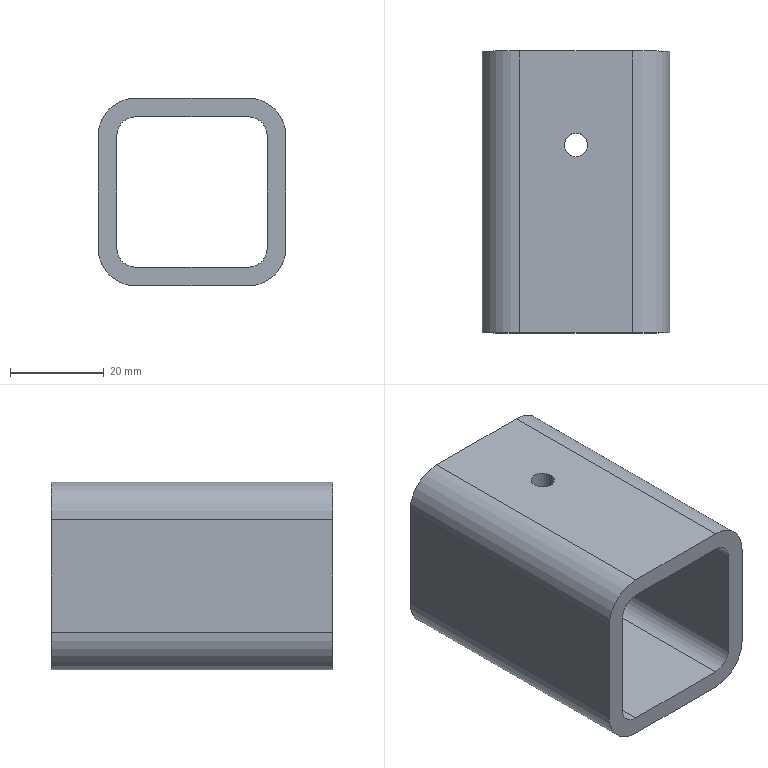Part | SolidWorks | features HoleWzd 1, WeldMemberFeat 1, WeldmentFeature 1 | 1 solid | 22 faces | box 40 x 60 x 40 mm | volume 31931 mm3 | cylinder 12 | plane 10 | commonest cylinder face diameters 5 x4 8 x4 16 x4
STEP:
#1=CARTESIAN_POINT('',(2.5,40.,16.));
#2=VERTEX_POINT('',#1);
#3=CARTESIAN_POINT('',(-2.5,40.,16.));
#4=VERTEX_POINT('',#3);
#5=CARTESIAN_POINT('',(0.,40.,16.));
#6=DIRECTION('',(0.,0.,-1.));
#7=DIRECTION('',(-1.,0.,0.));
#8=AXIS2_PLACEMENT_3D('',#5,#6,#7);
#9=CIRCLE('',#8,2.5);
#10=EDGE_CURVE('',#2,#4,#9,.T.);
#11=ORIENTED_EDGE('',*,*,#10,.T.);
#12=CARTESIAN_POINT('',(-2.5,40.,20.));
#13=VERTEX_POINT('',#12);
#14=CARTESIAN_POINT('',(-2.5,40.,20.));
#15=DIRECTION('',(0.,0.,1.));
#16=VECTOR('',#15,1000.);
#17=LINE('',#14,#16);
#18=EDGE_CURVE('',#4,#13,#17,.T.);
#19=ORIENTED_EDGE('',*,*,#18,.T.);
#20=CARTESIAN_POINT('',(2.5,40.,20.));
#21=VERTEX_POINT('',#20);
#22=CARTESIAN_POINT('',(0.,40.,20.));
#23=DIRECTION('',(0.,0.,1.));
#24=DIRECTION('',(1.,0.,0.));
#25=AXIS2_PLACEMENT_3D('',#22,#23,#24);
#26=CIRCLE('',#25,2.5);
#27=EDGE_CURVE('',#13,#21,#26,.T.);
#28=ORIENTED_EDGE('',*,*,#27,.T.);
#29=CARTESIAN_POINT('',(2.5,40.,20.));
#30=DIRECTION('',(0.,0.,1.));
#31=VECTOR('',#30,1000.);
#32=LINE('',#29,#31);
#33=EDGE_CURVE('',#2,#21,#32,.T.);
#34=ORIENTED_EDGE('',*,*,#33,.F.);
#35=EDGE_LOOP('',(#11,#19,#28,#34));
#36=FACE_OUTER_BOUND('',#35,.T.);
#37=CARTESIAN_POINT('',(0.,40.,20.));
#38=DIRECTION('',(0.,0.,1.));
#39=DIRECTION('',(1.,0.,0.));
#40=AXIS2_PLACEMENT_3D('',#37,#38,#39);
#41=CYLINDRICAL_SURFACE('',#40,2.5);
#42=ADVANCED_FACE('',(#36),#41,.F.);
#43=CARTESIAN_POINT('',(-2.5,40.,-20.));
#44=VERTEX_POINT('',#43);
#45=CARTESIAN_POINT('',(2.5,40.,-20.));
#46=VERTEX_POINT('',#45);
#47=CARTESIAN_POINT('',(0.,40.,-20.));
#48=DIRECTION('',(0.,0.,1.));
#49=DIRECTION('',(1.,0.,0.));
#50=AXIS2_PLACEMENT_3D('',#47,#48,#49);
#51=CIRCLE('',#50,2.5);
#52=EDGE_CURVE('',#44,#46,#51,.T.);
#53=ORIENTED_EDGE('',*,*,#52,.F.);
#54=CARTESIAN_POINT('',(-2.5,40.,-16.));
#55=VERTEX_POINT('',#54);
#56=CARTESIAN_POINT('',(-2.5,40.,20.));
#57=DIRECTION('',(0.,0.,1.));
#58=VECTOR('',#57,1000.);
#59=LINE('',#56,#58);
#60=EDGE_CURVE('',#44,#55,#59,.T.);
#61=ORIENTED_EDGE('',*,*,#60,.T.);
#62=CARTESIAN_POINT('',(2.5,40.,-16.));
#63=VERTEX_POINT('',#62);
#64=CARTESIAN_POINT('',(0.,40.,-16.));
#65=DIRECTION('',(0.,0.,1.));
#66=DIRECTION('',(1.,0.,0.));
#67=AXIS2_PLACEMENT_3D('',#64,#65,#66);
#68=CIRCLE('',#67,2.5);
#69=EDGE_CURVE('',#55,#63,#68,.T.);
#70=ORIENTED_EDGE('',*,*,#69,.T.);
#71=CARTESIAN_POINT('',(2.5,40.,20.));
#72=DIRECTION('',(0.,0.,1.));
#73=VECTOR('',#72,1000.);
#74=LINE('',#71,#73);
#75=EDGE_CURVE('',#46,#63,#74,.T.);
#76=ORIENTED_EDGE('',*,*,#75,.F.);
#77=EDGE_LOOP('',(#53,#61,#70,#76));
#78=FACE_OUTER_BOUND('',#77,.T.);
#79=CARTESIAN_POINT('',(0.,40.,20.));
#80=DIRECTION('',(0.,0.,1.));
#81=DIRECTION('',(1.,0.,0.));
#82=AXIS2_PLACEMENT_3D('',#79,#80,#81);
#83=CYLINDRICAL_SURFACE('',#82,2.5);
#84=ADVANCED_FACE('',(#78),#83,.F.);
#85=CARTESIAN_POINT('',(20.,60.,12.));
#86=VERTEX_POINT('',#85);
#87=CARTESIAN_POINT('',(12.,60.,20.));
#88=VERTEX_POINT('',#87);
#89=CARTESIAN_POINT('',(12.,60.,12.));
#90=DIRECTION('',(0.,-1.,0.));
#91=DIRECTION('',(1.,0.,0.));
#92=AXIS2_PLACEMENT_3D('',#89,#90,#91);
#93=CIRCLE('',#92,8.);
#94=EDGE_CURVE('',#86,#88,#93,.T.);
#95=ORIENTED_EDGE('',*,*,#94,.T.);
#96=CARTESIAN_POINT('',(12.,0.,20.));
#97=VERTEX_POINT('',#96);
#98=CARTESIAN_POINT('',(12.,0.,20.));
#99=DIRECTION('',(0.,1.,0.));
#100=VECTOR('',#99,1000.);
#101=LINE('',#98,#100);
#102=EDGE_CURVE('',#97,#88,#101,.T.);
#103=ORIENTED_EDGE('',*,*,#102,.F.);
#104=CARTESIAN_POINT('',(20.,0.,12.));
#105=VERTEX_POINT('',#104);
#106=CARTESIAN_POINT('',(12.,0.,12.));
#107=DIRECTION('',(0.,-1.,0.));
#108=DIRECTION('',(1.,0.,0.));
#109=AXIS2_PLACEMENT_3D('',#106,#107,#108);
#110=CIRCLE('',#109,8.);
#111=EDGE_CURVE('',#105,#97,#110,.T.);
#112=ORIENTED_EDGE('',*,*,#111,.F.);
#113=CARTESIAN_POINT('',(20.,0.,12.));
#114=DIRECTION('',(0.,1.,0.));
#115=VECTOR('',#114,1000.);
#116=LINE('',#113,#115);
#117=EDGE_CURVE('',#105,#86,#116,.T.);
#118=ORIENTED_EDGE('',*,*,#117,.T.);
#119=EDGE_LOOP('',(#95,#103,#112,#118));
#120=FACE_OUTER_BOUND('',#119,.T.);
#121=CARTESIAN_POINT('',(12.,0.,12.));
#122=DIRECTION('',(0.,1.,0.));
#123=DIRECTION('',(-1.,0.,0.));
#124=AXIS2_PLACEMENT_3D('',#121,#122,#123);
#125=CYLINDRICAL_SURFACE('',#124,8.);
#126=ADVANCED_FACE('',(#120),#125,.T.);
#127=CARTESIAN_POINT('',(0.,40.,20.));
#128=DIRECTION('',(0.,0.,1.));
#129=DIRECTION('',(1.,0.,0.));
#130=AXIS2_PLACEMENT_3D('',#127,#128,#129);
#131=CIRCLE('',#130,2.5);
#132=EDGE_CURVE('',#21,#13,#131,.T.);
#133=ORIENTED_EDGE('',*,*,#132,.F.);
#134=ORIENTED_EDGE('',*,*,#27,.F.);
#135=EDGE_LOOP('',(#133,#134));
#136=FACE_BOUND('',#135,.T.);
#137=CARTESIAN_POINT('',(-12.,60.,20.));
#138=VERTEX_POINT('',#137);
#139=CARTESIAN_POINT('',(12.,60.,20.));
#140=DIRECTION('',(-1.,0.,0.));
#141=VECTOR('',#140,1000.);
#142=LINE('',#139,#141);
#143=EDGE_CURVE('',#88,#138,#142,.T.);
#144=ORIENTED_EDGE('',*,*,#143,.T.);
#145=CARTESIAN_POINT('',(-12.,0.,20.));
#146=VERTEX_POINT('',#145);
#147=CARTESIAN_POINT('',(-12.,0.,20.));
#148=DIRECTION('',(0.,1.,0.));
#149=VECTOR('',#148,1000.);
#150=LINE('',#147,#149);
#151=EDGE_CURVE('',#146,#138,#150,.T.);
#152=ORIENTED_EDGE('',*,*,#151,.F.);
#153=CARTESIAN_POINT('',(12.,0.,20.));
#154=DIRECTION('',(-1.,0.,0.));
#155=VECTOR('',#154,1000.);
#156=LINE('',#153,#155);
#157=EDGE_CURVE('',#97,#146,#156,.T.);
#158=ORIENTED_EDGE('',*,*,#157,.F.);
#159=ORIENTED_EDGE('',*,*,#102,.T.);
#160=EDGE_LOOP('',(#144,#152,#158,#159));
#161=FACE_OUTER_BOUND('',#160,.T.);
#162=CARTESIAN_POINT('',(12.,0.,20.));
#163=DIRECTION('',(0.,0.,-1.));
#164=DIRECTION('',(-1.,0.,0.));
#165=AXIS2_PLACEMENT_3D('',#162,#163,#164);
#166=PLANE('',#165);
#167=ADVANCED_FACE('',(#136,#161),#166,.F.);
#168=CARTESIAN_POINT('',(-20.,60.,12.));
#169=VERTEX_POINT('',#168);
#170=CARTESIAN_POINT('',(-12.,60.,12.));
#171=DIRECTION('',(0.,-1.,0.));
#172=DIRECTION('',(1.,0.,0.));
#173=AXIS2_PLACEMENT_3D('',#170,#171,#172);
#174=CIRCLE('',#173,8.);
#175=EDGE_CURVE('',#138,#169,#174,.T.);
#176=ORIENTED_EDGE('',*,*,#175,.T.);
#177=CARTESIAN_POINT('',(-20.,0.,12.));
#178=VERTEX_POINT('',#177);
#179=CARTESIAN_POINT('',(-20.,0.,12.));
#180=DIRECTION('',(0.,1.,0.));
#181=VECTOR('',#180,1000.);
#182=LINE('',#179,#181);
#183=EDGE_CURVE('',#178,#169,#182,.T.);
#184=ORIENTED_EDGE('',*,*,#183,.F.);
#185=CARTESIAN_POINT('',(-12.,0.,12.));
#186=DIRECTION('',(0.,-1.,0.));
#187=DIRECTION('',(1.,0.,0.));
#188=AXIS2_PLACEMENT_3D('',#185,#186,#187);
#189=CIRCLE('',#188,8.);
#190=EDGE_CURVE('',#146,#178,#189,.T.);
#191=ORIENTED_EDGE('',*,*,#190,.F.);
#192=ORIENTED_EDGE('',*,*,#151,.T.);
#193=EDGE_LOOP('',(#176,#184,#191,#192));
#194=FACE_OUTER_BOUND('',#193,.T.);
#195=CARTESIAN_POINT('',(-12.,0.,12.));
#196=DIRECTION('',(0.,1.,0.));
#197=DIRECTION('',(-1.,0.,0.));
#198=AXIS2_PLACEMENT_3D('',#195,#196,#197);
#199=CYLINDRICAL_SURFACE('',#198,8.);
#200=ADVANCED_FACE('',(#194),#199,.T.);
#201=CARTESIAN_POINT('',(-20.,60.,-12.));
#202=VERTEX_POINT('',#201);
#203=CARTESIAN_POINT('',(-20.,60.,-12.));
#204=DIRECTION('',(0.,0.,-1.));
#205=VECTOR('',#204,1000.);
#206=LINE('',#203,#205);
#207=EDGE_CURVE('',#169,#202,#206,.T.);
#208=ORIENTED_EDGE('',*,*,#207,.T.);
#209=CARTESIAN_POINT('',(-20.,0.,-12.));
#210=VERTEX_POINT('',#209);
#211=CARTESIAN_POINT('',(-20.,0.,-12.));
#212=DIRECTION('',(0.,1.,0.));
#213=VECTOR('',#212,1000.);
#214=LINE('',#211,#213);
#215=EDGE_CURVE('',#210,#202,#214,.T.);
#216=ORIENTED_EDGE('',*,*,#215,.F.);
#217=CARTESIAN_POINT('',(-20.,0.,-12.));
#218=DIRECTION('',(0.,0.,-1.));
#219=VECTOR('',#218,1000.);
#220=LINE('',#217,#219);
#221=EDGE_CURVE('',#178,#210,#220,.T.);
#222=ORIENTED_EDGE('',*,*,#221,.F.);
#223=ORIENTED_EDGE('',*,*,#183,.T.);
#224=EDGE_LOOP('',(#208,#216,#222,#223));
#225=FACE_OUTER_BOUND('',#224,.T.);
#226=CARTESIAN_POINT('',(-20.,0.,-12.));
#227=DIRECTION('',(1.,0.,0.));
#228=DIRECTION('',(0.,1.,0.));
#229=AXIS2_PLACEMENT_3D('',#226,#227,#228);
#230=PLANE('',#229);
#231=ADVANCED_FACE('',(#225),#230,.F.);
#232=CARTESIAN_POINT('',(-12.,60.,-20.));
#233=VERTEX_POINT('',#232);
#234=CARTESIAN_POINT('',(-12.,60.,-12.));
#235=DIRECTION('',(0.,-1.,0.));
#236=DIRECTION('',(1.,0.,0.));
#237=AXIS2_PLACEMENT_3D('',#234,#235,#236);
#238=CIRCLE('',#237,8.);
#239=EDGE_CURVE('',#202,#233,#238,.T.);
#240=ORIENTED_EDGE('',*,*,#239,.T.);
#241=CARTESIAN_POINT('',(-12.,0.,-20.));
#242=VERTEX_POINT('',#241);
#243=CARTESIAN_POINT('',(-12.,0.,-20.));
#244=DIRECTION('',(0.,1.,0.));
#245=VECTOR('',#244,1000.);
#246=LINE('',#243,#245);
#247=EDGE_CURVE('',#242,#233,#246,.T.);
#248=ORIENTED_EDGE('',*,*,#247,.F.);
#249=CARTESIAN_POINT('',(-12.,0.,-12.));
#250=DIRECTION('',(0.,-1.,0.));
#251=DIRECTION('',(1.,0.,0.));
#252=AXIS2_PLACEMENT_3D('',#249,#250,#251);
#253=CIRCLE('',#252,8.);
#254=EDGE_CURVE('',#210,#242,#253,.T.);
#255=ORIENTED_EDGE('',*,*,#254,.F.);
#256=ORIENTED_EDGE('',*,*,#215,.T.);
#257=EDGE_LOOP('',(#240,#248,#255,#256));
#258=FACE_OUTER_BOUND('',#257,.T.);
#259=CARTESIAN_POINT('',(-12.,0.,-12.));
#260=DIRECTION('',(0.,1.,0.));
#261=DIRECTION('',(-1.,0.,0.));
#262=AXIS2_PLACEMENT_3D('',#259,#260,#261);
#263=CYLINDRICAL_SURFACE('',#262,8.);
#264=ADVANCED_FACE('',(#258),#263,.T.);
#265=CARTESIAN_POINT('',(0.,40.,-20.));
#266=DIRECTION('',(0.,0.,1.));
#267=DIRECTION('',(1.,0.,0.));
#268=AXIS2_PLACEMENT_3D('',#265,#266,#267);
#269=CIRCLE('',#268,2.5);
#270=EDGE_CURVE('',#46,#44,#269,.T.);
#271=ORIENTED_EDGE('',*,*,#270,.T.);
#272=ORIENTED_EDGE('',*,*,#52,.T.);
#273=EDGE_LOOP('',(#271,#272));
#274=FACE_BOUND('',#273,.T.);
#275=CARTESIAN_POINT('',(12.,60.,-20.));
#276=VERTEX_POINT('',#275);
#277=CARTESIAN_POINT('',(-12.,60.,-20.));
#278=DIRECTION('',(1.,0.,0.));
#279=VECTOR('',#278,1000.);
#280=LINE('',#277,#279);
#281=EDGE_CURVE('',#233,#276,#280,.T.);
#282=ORIENTED_EDGE('',*,*,#281,.T.);
#283=CARTESIAN_POINT('',(12.,0.,-20.));
#284=VERTEX_POINT('',#283);
#285=CARTESIAN_POINT('',(12.,0.,-20.));
#286=DIRECTION('',(0.,1.,0.));
#287=VECTOR('',#286,1000.);
#288=LINE('',#285,#287);
#289=EDGE_CURVE('',#284,#276,#288,.T.);
#290=ORIENTED_EDGE('',*,*,#289,.F.);
#291=CARTESIAN_POINT('',(-12.,0.,-20.));
#292=DIRECTION('',(1.,0.,0.));
#293=VECTOR('',#292,1000.);
#294=LINE('',#291,#293);
#295=EDGE_CURVE('',#242,#284,#294,.T.);
#296=ORIENTED_EDGE('',*,*,#295,.F.);
#297=ORIENTED_EDGE('',*,*,#247,.T.);
#298=EDGE_LOOP('',(#282,#290,#296,#297));
#299=FACE_OUTER_BOUND('',#298,.T.);
#300=CARTESIAN_POINT('',(-12.,0.,-20.));
#301=DIRECTION('',(0.,0.,1.));
#302=DIRECTION('',(1.,0.,0.));
#303=AXIS2_PLACEMENT_3D('',#300,#301,#302);
#304=PLANE('',#303);
#305=ADVANCED_FACE('',(#274,#299),#304,.F.);
#306=CARTESIAN_POINT('',(20.,60.,-12.));
#307=VERTEX_POINT('',#306);
#308=CARTESIAN_POINT('',(12.,60.,-12.));
#309=DIRECTION('',(0.,-1.,0.));
#310=DIRECTION('',(1.,0.,0.));
#311=AXIS2_PLACEMENT_3D('',#308,#309,#310);
#312=CIRCLE('',#311,8.);
#313=EDGE_CURVE('',#276,#307,#312,.T.);
#314=ORIENTED_EDGE('',*,*,#313,.T.);
#315=CARTESIAN_POINT('',(20.,0.,-12.));
#316=VERTEX_POINT('',#315);
#317=CARTESIAN_POINT('',(20.,0.,-12.));
#318=DIRECTION('',(0.,1.,0.));
#319=VECTOR('',#318,1000.);
#320=LINE('',#317,#319);
#321=EDGE_CURVE('',#316,#307,#320,.T.);
#322=ORIENTED_EDGE('',*,*,#321,.F.);
#323=CARTESIAN_POINT('',(12.,0.,-12.));
#324=DIRECTION('',(0.,-1.,0.));
#325=DIRECTION('',(1.,0.,0.));
#326=AXIS2_PLACEMENT_3D('',#323,#324,#325);
#327=CIRCLE('',#326,8.);
#328=EDGE_CURVE('',#284,#316,#327,.T.);
#329=ORIENTED_EDGE('',*,*,#328,.F.);
#330=ORIENTED_EDGE('',*,*,#289,.T.);
#331=EDGE_LOOP('',(#314,#322,#329,#330));
#332=FACE_OUTER_BOUND('',#331,.T.);
#333=CARTESIAN_POINT('',(12.,0.,-12.));
#334=DIRECTION('',(0.,1.,0.));
#335=DIRECTION('',(-1.,0.,0.));
#336=AXIS2_PLACEMENT_3D('',#333,#334,#335);
#337=CYLINDRICAL_SURFACE('',#336,8.);
#338=ADVANCED_FACE('',(#332),#337,.T.);
#339=CARTESIAN_POINT('',(-12.,60.,16.));
#340=VERTEX_POINT('',#339);
#341=CARTESIAN_POINT('',(-16.,60.,12.));
#342=VERTEX_POINT('',#341);
#343=CARTESIAN_POINT('',(-12.,60.,12.));
#344=DIRECTION('',(0.,-1.,0.));
#345=DIRECTION('',(1.,0.,0.));
#346=AXIS2_PLACEMENT_3D('',#343,#344,#345);
#347=CIRCLE('',#346,4.);
#348=EDGE_CURVE('',#340,#342,#347,.T.);
#349=ORIENTED_EDGE('',*,*,#348,.F.);
#350=CARTESIAN_POINT('',(-12.,0.,16.));
#351=VERTEX_POINT('',#350);
#352=CARTESIAN_POINT('',(-12.,0.,16.));
#353=DIRECTION('',(0.,1.,0.));
#354=VECTOR('',#353,1000.);
#355=LINE('',#352,#354);
#356=EDGE_CURVE('',#351,#340,#355,.T.);
#357=ORIENTED_EDGE('',*,*,#356,.F.);
#358=CARTESIAN_POINT('',(-16.,0.,12.));
#359=VERTEX_POINT('',#358);
#360=CARTESIAN_POINT('',(-12.,0.,12.));
#361=DIRECTION('',(0.,-1.,0.));
#362=DIRECTION('',(1.,0.,0.));
#363=AXIS2_PLACEMENT_3D('',#360,#361,#362);
#364=CIRCLE('',#363,4.);
#365=EDGE_CURVE('',#351,#359,#364,.T.);
#366=ORIENTED_EDGE('',*,*,#365,.T.);
#367=CARTESIAN_POINT('',(-16.,0.,12.));
#368=DIRECTION('',(0.,1.,0.));
#369=VECTOR('',#368,1000.);
#370=LINE('',#367,#369);
#371=EDGE_CURVE('',#359,#342,#370,.T.);
#372=ORIENTED_EDGE('',*,*,#371,.T.);
#373=EDGE_LOOP('',(#349,#357,#366,#372));
#374=FACE_OUTER_BOUND('',#373,.T.);
#375=CARTESIAN_POINT('',(-12.,0.,12.));
#376=DIRECTION('',(0.,1.,0.));
#377=DIRECTION('',(-1.,0.,0.));
#378=AXIS2_PLACEMENT_3D('',#375,#376,#377);
#379=CYLINDRICAL_SURFACE('',#378,4.);
#380=ADVANCED_FACE('',(#374),#379,.F.);
#381=ORIENTED_EDGE('',*,*,#10,.F.);
#382=CARTESIAN_POINT('',(0.,40.,16.));
#383=DIRECTION('',(0.,0.,-1.));
#384=DIRECTION('',(-1.,0.,0.));
#385=AXIS2_PLACEMENT_3D('',#382,#383,#384);
#386=CIRCLE('',#385,2.5);
#387=EDGE_CURVE('',#4,#2,#386,.T.);
#388=ORIENTED_EDGE('',*,*,#387,.F.);
#389=EDGE_LOOP('',(#381,#388));
#390=FACE_BOUND('',#389,.T.);
#391=CARTESIAN_POINT('',(12.,60.,16.));
#392=VERTEX_POINT('',#391);
#393=CARTESIAN_POINT('',(12.,60.,16.));
#394=DIRECTION('',(-1.,0.,0.));
#395=VECTOR('',#394,1000.);
#396=LINE('',#393,#395);
#397=EDGE_CURVE('',#392,#340,#396,.T.);
#398=ORIENTED_EDGE('',*,*,#397,.F.);
#399=CARTESIAN_POINT('',(12.,0.,16.));
#400=VERTEX_POINT('',#399);
#401=CARTESIAN_POINT('',(12.,0.,16.));
#402=DIRECTION('',(0.,1.,0.));
#403=VECTOR('',#402,1000.);
#404=LINE('',#401,#403);
#405=EDGE_CURVE('',#400,#392,#404,.T.);
#406=ORIENTED_EDGE('',*,*,#405,.F.);
#407=CARTESIAN_POINT('',(12.,0.,16.));
#408=DIRECTION('',(-1.,0.,0.));
#409=VECTOR('',#408,1000.);
#410=LINE('',#407,#409);
#411=EDGE_CURVE('',#400,#351,#410,.T.);
#412=ORIENTED_EDGE('',*,*,#411,.T.);
#413=ORIENTED_EDGE('',*,*,#356,.T.);
#414=EDGE_LOOP('',(#398,#406,#412,#413));
#415=FACE_OUTER_BOUND('',#414,.T.);
#416=CARTESIAN_POINT('',(12.,0.,16.));
#417=DIRECTION('',(0.,0.,-1.));
#418=DIRECTION('',(-1.,0.,0.));
#419=AXIS2_PLACEMENT_3D('',#416,#417,#418);
#420=PLANE('',#419);
#421=ADVANCED_FACE('',(#390,#415),#420,.T.);
#422=CARTESIAN_POINT('',(16.,60.,12.));
#423=VERTEX_POINT('',#422);
#424=CARTESIAN_POINT('',(12.,60.,12.));
#425=DIRECTION('',(0.,-1.,0.));
#426=DIRECTION('',(1.,0.,0.));
#427=AXIS2_PLACEMENT_3D('',#424,#425,#426);
#428=CIRCLE('',#427,4.);
#429=EDGE_CURVE('',#423,#392,#428,.T.);
#430=ORIENTED_EDGE('',*,*,#429,.F.);
#431=CARTESIAN_POINT('',(16.,0.,12.));
#432=VERTEX_POINT('',#431);
#433=CARTESIAN_POINT('',(16.,0.,12.));
#434=DIRECTION('',(0.,1.,0.));
#435=VECTOR('',#434,1000.);
#436=LINE('',#433,#435);
#437=EDGE_CURVE('',#432,#423,#436,.T.);
#438=ORIENTED_EDGE('',*,*,#437,.F.);
#439=CARTESIAN_POINT('',(12.,0.,12.));
#440=DIRECTION('',(0.,-1.,0.));
#441=DIRECTION('',(1.,0.,0.));
#442=AXIS2_PLACEMENT_3D('',#439,#440,#441);
#443=CIRCLE('',#442,4.);
#444=EDGE_CURVE('',#432,#400,#443,.T.);
#445=ORIENTED_EDGE('',*,*,#444,.T.);
#446=ORIENTED_EDGE('',*,*,#405,.T.);
#447=EDGE_LOOP('',(#430,#438,#445,#446));
#448=FACE_OUTER_BOUND('',#447,.T.);
#449=CARTESIAN_POINT('',(12.,0.,12.));
#450=DIRECTION('',(0.,1.,0.));
#451=DIRECTION('',(-1.,0.,0.));
#452=AXIS2_PLACEMENT_3D('',#449,#450,#451);
#453=CYLINDRICAL_SURFACE('',#452,4.);
#454=ADVANCED_FACE('',(#448),#453,.F.);
#455=CARTESIAN_POINT('',(16.,60.,-12.));
#456=VERTEX_POINT('',#455);
#457=CARTESIAN_POINT('',(16.,60.,12.));
#458=DIRECTION('',(0.,0.,1.));
#459=VECTOR('',#458,1000.);
#460=LINE('',#457,#459);
#461=EDGE_CURVE('',#456,#423,#460,.T.);
#462=ORIENTED_EDGE('',*,*,#461,.F.);
#463=CARTESIAN_POINT('',(16.,0.,-12.));
#464=VERTEX_POINT('',#463);
#465=CARTESIAN_POINT('',(16.,0.,-12.));
#466=DIRECTION('',(0.,1.,0.));
#467=VECTOR('',#466,1000.);
#468=LINE('',#465,#467);
#469=EDGE_CURVE('',#464,#456,#468,.T.);
#470=ORIENTED_EDGE('',*,*,#469,.F.);
#471=CARTESIAN_POINT('',(16.,0.,12.));
#472=DIRECTION('',(0.,0.,1.));
#473=VECTOR('',#472,1000.);
#474=LINE('',#471,#473);
#475=EDGE_CURVE('',#464,#432,#474,.T.);
#476=ORIENTED_EDGE('',*,*,#475,.T.);
#477=ORIENTED_EDGE('',*,*,#437,.T.);
#478=EDGE_LOOP('',(#462,#470,#476,#477));
#479=FACE_OUTER_BOUND('',#478,.T.);
#480=CARTESIAN_POINT('',(16.,0.,12.));
#481=DIRECTION('',(-1.,0.,0.));
#482=DIRECTION('',(0.,-1.,0.));
#483=AXIS2_PLACEMENT_3D('',#480,#481,#482);
#484=PLANE('',#483);
#485=ADVANCED_FACE('',(#479),#484,.T.);
#486=CARTESIAN_POINT('',(12.,60.,-16.));
#487=VERTEX_POINT('',#486);
#488=CARTESIAN_POINT('',(12.,60.,-12.));
#489=DIRECTION('',(0.,-1.,0.));
#490=DIRECTION('',(1.,0.,0.));
#491=AXIS2_PLACEMENT_3D('',#488,#489,#490);
#492=CIRCLE('',#491,4.);
#493=EDGE_CURVE('',#487,#456,#492,.T.);
#494=ORIENTED_EDGE('',*,*,#493,.F.);
#495=CARTESIAN_POINT('',(12.,0.,-16.));
#496=VERTEX_POINT('',#495);
#497=CARTESIAN_POINT('',(12.,0.,-16.));
#498=DIRECTION('',(0.,1.,0.));
#499=VECTOR('',#498,1000.);
#500=LINE('',#497,#499);
#501=EDGE_CURVE('',#496,#487,#500,.T.);
#502=ORIENTED_EDGE('',*,*,#501,.F.);
#503=CARTESIAN_POINT('',(12.,0.,-12.));
#504=DIRECTION('',(0.,-1.,0.));
#505=DIRECTION('',(1.,0.,0.));
#506=AXIS2_PLACEMENT_3D('',#503,#504,#505);
#507=CIRCLE('',#506,4.);
#508=EDGE_CURVE('',#496,#464,#507,.T.);
#509=ORIENTED_EDGE('',*,*,#508,.T.);
#510=ORIENTED_EDGE('',*,*,#469,.T.);
#511=EDGE_LOOP('',(#494,#502,#509,#510));
#512=FACE_OUTER_BOUND('',#511,.T.);
#513=CARTESIAN_POINT('',(12.,0.,-12.));
#514=DIRECTION('',(0.,1.,0.));
#515=DIRECTION('',(-1.,0.,0.));
#516=AXIS2_PLACEMENT_3D('',#513,#514,#515);
#517=CYLINDRICAL_SURFACE('',#516,4.);
#518=ADVANCED_FACE('',(#512),#517,.F.);
#519=CARTESIAN_POINT('',(0.,40.,-16.));
#520=DIRECTION('',(0.,0.,1.));
#521=DIRECTION('',(1.,0.,0.));
#522=AXIS2_PLACEMENT_3D('',#519,#520,#521);
#523=CIRCLE('',#522,2.5);
#524=EDGE_CURVE('',#63,#55,#523,.T.);
#525=ORIENTED_EDGE('',*,*,#524,.F.);
#526=ORIENTED_EDGE('',*,*,#69,.F.);
#527=EDGE_LOOP('',(#525,#526));
#528=FACE_BOUND('',#527,.T.);
#529=CARTESIAN_POINT('',(-12.,60.,-16.));
#530=VERTEX_POINT('',#529);
#531=CARTESIAN_POINT('',(-12.,60.,-16.));
#532=DIRECTION('',(1.,0.,0.));
#533=VECTOR('',#532,1000.);
#534=LINE('',#531,#533);
#535=EDGE_CURVE('',#530,#487,#534,.T.);
#536=ORIENTED_EDGE('',*,*,#535,.F.);
#537=CARTESIAN_POINT('',(-12.,0.,-16.));
#538=VERTEX_POINT('',#537);
#539=CARTESIAN_POINT('',(-12.,0.,-16.));
#540=DIRECTION('',(0.,1.,0.));
#541=VECTOR('',#540,1000.);
#542=LINE('',#539,#541);
#543=EDGE_CURVE('',#538,#530,#542,.T.);
#544=ORIENTED_EDGE('',*,*,#543,.F.);
#545=CARTESIAN_POINT('',(-12.,0.,-16.));
#546=DIRECTION('',(1.,0.,0.));
#547=VECTOR('',#546,1000.);
#548=LINE('',#545,#547);
#549=EDGE_CURVE('',#538,#496,#548,.T.);
#550=ORIENTED_EDGE('',*,*,#549,.T.);
#551=ORIENTED_EDGE('',*,*,#501,.T.);
#552=EDGE_LOOP('',(#536,#544,#550,#551));
#553=FACE_OUTER_BOUND('',#552,.T.);
#554=CARTESIAN_POINT('',(-12.,0.,-16.));
#555=DIRECTION('',(0.,0.,1.));
#556=DIRECTION('',(1.,0.,0.));
#557=AXIS2_PLACEMENT_3D('',#554,#555,#556);
#558=PLANE('',#557);
#559=ADVANCED_FACE('',(#528,#553),#558,.T.);
#560=CARTESIAN_POINT('',(-16.,60.,-12.));
#561=VERTEX_POINT('',#560);
#562=CARTESIAN_POINT('',(-12.,60.,-12.));
#563=DIRECTION('',(0.,-1.,0.));
#564=DIRECTION('',(1.,0.,0.));
#565=AXIS2_PLACEMENT_3D('',#562,#563,#564);
#566=CIRCLE('',#565,4.);
#567=EDGE_CURVE('',#561,#530,#566,.T.);
#568=ORIENTED_EDGE('',*,*,#567,.F.);
#569=CARTESIAN_POINT('',(-16.,0.,-12.));
#570=VERTEX_POINT('',#569);
#571=CARTESIAN_POINT('',(-16.,0.,-12.));
#572=DIRECTION('',(0.,1.,0.));
#573=VECTOR('',#572,1000.);
#574=LINE('',#571,#573);
#575=EDGE_CURVE('',#570,#561,#574,.T.);
#576=ORIENTED_EDGE('',*,*,#575,.F.);
#577=CARTESIAN_POINT('',(-12.,0.,-12.));
#578=DIRECTION('',(0.,-1.,0.));
#579=DIRECTION('',(1.,0.,0.));
#580=AXIS2_PLACEMENT_3D('',#577,#578,#579);
#581=CIRCLE('',#580,4.);
#582=EDGE_CURVE('',#570,#538,#581,.T.);
#583=ORIENTED_EDGE('',*,*,#582,.T.);
#584=ORIENTED_EDGE('',*,*,#543,.T.);
#585=EDGE_LOOP('',(#568,#576,#583,#584));
#586=FACE_OUTER_BOUND('',#585,.T.);
#587=CARTESIAN_POINT('',(-12.,0.,-12.));
#588=DIRECTION('',(0.,1.,0.));
#589=DIRECTION('',(-1.,0.,0.));
#590=AXIS2_PLACEMENT_3D('',#587,#588,#589);
#591=CYLINDRICAL_SURFACE('',#590,4.);
#592=ADVANCED_FACE('',(#586),#591,.F.);
#593=CARTESIAN_POINT('',(-16.,60.,-12.));
#594=DIRECTION('',(0.,0.,-1.));
#595=VECTOR('',#594,1000.);
#596=LINE('',#593,#595);
#597=EDGE_CURVE('',#342,#561,#596,.T.);
#598=ORIENTED_EDGE('',*,*,#597,.F.);
#599=ORIENTED_EDGE('',*,*,#371,.F.);
#600=CARTESIAN_POINT('',(-16.,0.,-12.));
#601=DIRECTION('',(0.,0.,-1.));
#602=VECTOR('',#601,1000.);
#603=LINE('',#600,#602);
#604=EDGE_CURVE('',#359,#570,#603,.T.);
#605=ORIENTED_EDGE('',*,*,#604,.T.);
#606=ORIENTED_EDGE('',*,*,#575,.T.);
#607=EDGE_LOOP('',(#598,#599,#605,#606));
#608=FACE_OUTER_BOUND('',#607,.T.);
#609=CARTESIAN_POINT('',(-16.,0.,-12.));
#610=DIRECTION('',(1.,0.,0.));
#611=DIRECTION('',(0.,1.,0.));
#612=AXIS2_PLACEMENT_3D('',#609,#610,#611);
#613=PLANE('',#612);
#614=ADVANCED_FACE('',(#608),#613,.T.);
#615=CARTESIAN_POINT('',(20.,60.,12.));
#616=DIRECTION('',(0.,0.,1.));
#617=VECTOR('',#616,1000.);
#618=LINE('',#615,#617);
#619=EDGE_CURVE('',#307,#86,#618,.T.);
#620=ORIENTED_EDGE('',*,*,#619,.T.);
#621=ORIENTED_EDGE('',*,*,#117,.F.);
#622=CARTESIAN_POINT('',(20.,0.,12.));
#623=DIRECTION('',(0.,0.,1.));
#624=VECTOR('',#623,1000.);
#625=LINE('',#622,#624);
#626=EDGE_CURVE('',#316,#105,#625,.T.);
#627=ORIENTED_EDGE('',*,*,#626,.F.);
#628=ORIENTED_EDGE('',*,*,#321,.T.);
#629=EDGE_LOOP('',(#620,#621,#627,#628));
#630=FACE_OUTER_BOUND('',#629,.T.);
#631=CARTESIAN_POINT('',(20.,0.,12.));
#632=DIRECTION('',(-1.,0.,0.));
#633=DIRECTION('',(0.,-1.,0.));
#634=AXIS2_PLACEMENT_3D('',#631,#632,#633);
#635=PLANE('',#634);
#636=ADVANCED_FACE('',(#630),#635,.F.);
#637=ORIENTED_EDGE('',*,*,#365,.F.);
#638=ORIENTED_EDGE('',*,*,#411,.F.);
#639=ORIENTED_EDGE('',*,*,#444,.F.);
#640=ORIENTED_EDGE('',*,*,#475,.F.);
#641=ORIENTED_EDGE('',*,*,#508,.F.);
#642=ORIENTED_EDGE('',*,*,#549,.F.);
#643=ORIENTED_EDGE('',*,*,#582,.F.);
#644=ORIENTED_EDGE('',*,*,#604,.F.);
#645=EDGE_LOOP('',(#637,#638,#639,#640,#641,#642,#643,#644));
#646=FACE_BOUND('',#645,.T.);
#647=ORIENTED_EDGE('',*,*,#111,.T.);
#648=ORIENTED_EDGE('',*,*,#157,.T.);
#649=ORIENTED_EDGE('',*,*,#190,.T.);
#650=ORIENTED_EDGE('',*,*,#221,.T.);
#651=ORIENTED_EDGE('',*,*,#254,.T.);
#652=ORIENTED_EDGE('',*,*,#295,.T.);
#653=ORIENTED_EDGE('',*,*,#328,.T.);
#654=ORIENTED_EDGE('',*,*,#626,.T.);
#655=EDGE_LOOP('',(#647,#648,#649,#650,#651,#652,#653,#654));
#656=FACE_OUTER_BOUND('',#655,.T.);
#657=CARTESIAN_POINT('',(12.,0.,12.));
#658=DIRECTION('',(0.,-1.,0.));
#659=DIRECTION('',(1.,0.,0.));
#660=AXIS2_PLACEMENT_3D('',#657,#658,#659);
#661=PLANE('',#660);
#662=ADVANCED_FACE('',(#646,#656),#661,.T.);
#663=ORIENTED_EDGE('',*,*,#348,.T.);
#664=ORIENTED_EDGE('',*,*,#597,.T.);
#665=ORIENTED_EDGE('',*,*,#567,.T.);
#666=ORIENTED_EDGE('',*,*,#535,.T.);
#667=ORIENTED_EDGE('',*,*,#493,.T.);
#668=ORIENTED_EDGE('',*,*,#461,.T.);
#669=ORIENTED_EDGE('',*,*,#429,.T.);
#670=ORIENTED_EDGE('',*,*,#397,.T.);
#671=EDGE_LOOP('',(#663,#664,#665,#666,#667,#668,#669,#670));
#672=FACE_BOUND('',#671,.T.);
#673=ORIENTED_EDGE('',*,*,#94,.F.);
#674=ORIENTED_EDGE('',*,*,#619,.F.);
#675=ORIENTED_EDGE('',*,*,#313,.F.);
#676=ORIENTED_EDGE('',*,*,#281,.F.);
#677=ORIENTED_EDGE('',*,*,#239,.F.);
#678=ORIENTED_EDGE('',*,*,#207,.F.);
#679=ORIENTED_EDGE('',*,*,#175,.F.);
#680=ORIENTED_EDGE('',*,*,#143,.F.);
#681=EDGE_LOOP('',(#673,#674,#675,#676,#677,#678,#679,#680));
#682=FACE_OUTER_BOUND('',#681,.T.);
#683=CARTESIAN_POINT('',(12.,60.,12.));
#684=DIRECTION('',(0.,-1.,0.));
#685=DIRECTION('',(1.,0.,0.));
#686=AXIS2_PLACEMENT_3D('',#683,#684,#685);
#687=PLANE('',#686);
#688=ADVANCED_FACE('',(#672,#682),#687,.F.);
#689=ORIENTED_EDGE('',*,*,#60,.F.);
#690=ORIENTED_EDGE('',*,*,#270,.F.);
#691=ORIENTED_EDGE('',*,*,#75,.T.);
#692=ORIENTED_EDGE('',*,*,#524,.T.);
#693=EDGE_LOOP('',(#689,#690,#691,#692));
#694=FACE_OUTER_BOUND('',#693,.T.);
#695=CARTESIAN_POINT('',(0.,40.,20.));
#696=DIRECTION('',(0.,0.,1.));
#697=DIRECTION('',(1.,0.,0.));
#698=AXIS2_PLACEMENT_3D('',#695,#696,#697);
#699=CYLINDRICAL_SURFACE('',#698,2.5);
#700=ADVANCED_FACE('',(#694),#699,.F.);
#701=ORIENTED_EDGE('',*,*,#18,.F.);
#702=ORIENTED_EDGE('',*,*,#387,.T.);
#703=ORIENTED_EDGE('',*,*,#33,.T.);
#704=ORIENTED_EDGE('',*,*,#132,.T.);
#705=EDGE_LOOP('',(#701,#702,#703,#704));
#706=FACE_OUTER_BOUND('',#705,.T.);
#707=CARTESIAN_POINT('',(0.,40.,20.));
#708=DIRECTION('',(0.,0.,1.));
#709=DIRECTION('',(1.,0.,0.));
#710=AXIS2_PLACEMENT_3D('',#707,#708,#709);
#711=CYLINDRICAL_SURFACE('',#710,2.5);
#712=ADVANCED_FACE('',(#706),#711,.F.);
#713=CLOSED_SHELL('',(#42,#84,#126,#167,#200,#231,#264,#305,#338,#380,#421,#454,#485,#518,#559,#592,#614,#636,#662,#688,#700,#712));
#714=MANIFOLD_SOLID_BREP('',#713);
#715=CARTESIAN_POINT('',(0.,0.,0.));
#716=DIRECTION('',(0.,0.,1.));
#717=DIRECTION('',(1.,0.,0.));
#718=AXIS2_PLACEMENT_3D('',#715,#716,#717);
#719=(LENGTH_UNIT()NAMED_UNIT(*)SI_UNIT(.MILLI.,.METRE.));
#720=UNCERTAINTY_MEASURE_WITH_UNIT(LENGTH_MEASURE(0.00001),#719,'','');
#721=(NAMED_UNIT(*)PLANE_ANGLE_UNIT()SI_UNIT($,.RADIAN.));
#722=(NAMED_UNIT(*)SI_UNIT($,.STERADIAN.)SOLID_ANGLE_UNIT());
#723=(GEOMETRIC_REPRESENTATION_CONTEXT(3)GLOBAL_UNCERTAINTY_ASSIGNED_CONTEXT((#720))GLOBAL_UNIT_ASSIGNED_CONTEXT((#719,#721,#722))REPRESENTATION_CONTEXT('',''));
#724=ADVANCED_BREP_SHAPE_REPRESENTATION('',(#714,#718),#723);